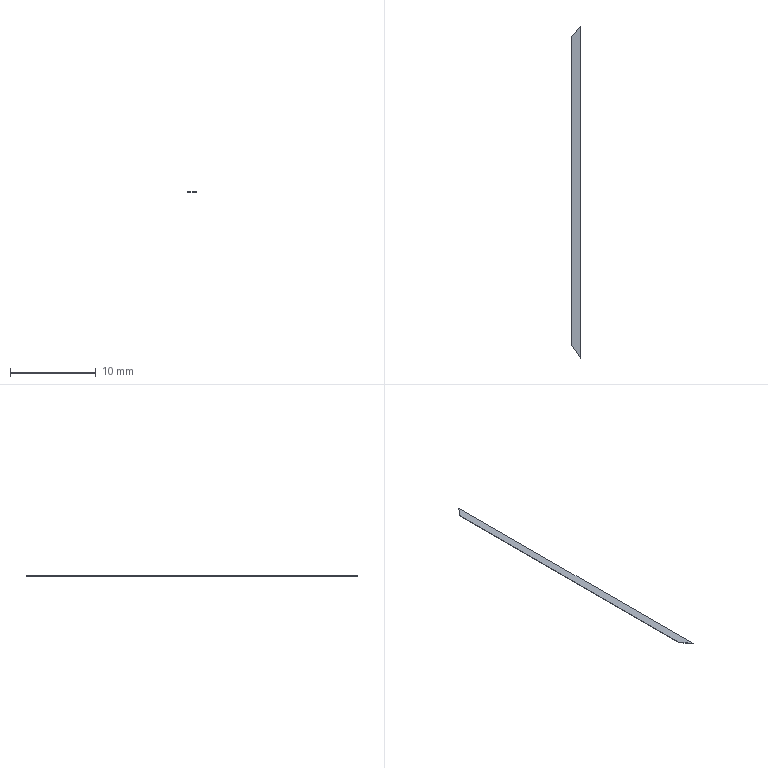Part | NX | features DATUM_CSYS 2, EXTRUDE 1, SKETCH 1 | 1 solid | 6 faces | box 1 x 38.63 x 0.05 mm | volume 1.865 mm3 | plane 6
STEP:
#1=CARTESIAN_POINT('',(0.,35.96,0.));
#2=VERTEX_POINT('',#1);
#3=CARTESIAN_POINT('',(0.,0.,0.));
#4=VERTEX_POINT('',#3);
#5=CARTESIAN_POINT('',(0.,35.96,0.));
#6=DIRECTION('',(0.,-1.,0.));
#7=VECTOR('',#6,1000.);
#8=LINE('',#5,#7);
#9=EDGE_CURVE('',#2,#4,#8,.T.);
#10=ORIENTED_EDGE('',*,*,#9,.T.);
#11=CARTESIAN_POINT('',(0.,0.,0.05));
#12=VERTEX_POINT('',#11);
#13=CARTESIAN_POINT('',(0.,0.,0.05));
#14=DIRECTION('',(0.,0.,-1.));
#15=VECTOR('',#14,1000.);
#16=LINE('',#13,#15);
#17=EDGE_CURVE('',#12,#4,#16,.T.);
#18=ORIENTED_EDGE('',*,*,#17,.F.);
#19=CARTESIAN_POINT('',(0.,35.96,0.05));
#20=VERTEX_POINT('',#19);
#21=CARTESIAN_POINT('',(0.,35.96,0.05));
#22=DIRECTION('',(0.,-1.,0.));
#23=VECTOR('',#22,1000.);
#24=LINE('',#21,#23);
#25=EDGE_CURVE('',#20,#12,#24,.T.);
#26=ORIENTED_EDGE('',*,*,#25,.F.);
#27=CARTESIAN_POINT('',(0.,35.96,0.05));
#28=DIRECTION('',(0.,0.,-1.));
#29=VECTOR('',#28,1000.);
#30=LINE('',#27,#29);
#31=EDGE_CURVE('',#20,#2,#30,.T.);
#32=ORIENTED_EDGE('',*,*,#31,.T.);
#33=EDGE_LOOP('',(#10,#18,#26,#32));
#34=FACE_BOUND('',#33,.T.);
#35=CARTESIAN_POINT('',(0.,35.96,0.05));
#36=DIRECTION('',(1.,0.,0.));
#37=DIRECTION('',(0.,0.,-1.));
#38=AXIS2_PLACEMENT_3D('',#35,#36,#37);
#39=PLANE('',#38);
#40=ADVANCED_FACE('',(#34),#39,.F.);
#41=CARTESIAN_POINT('',(1.,-1.41,0.));
#42=VERTEX_POINT('',#41);
#43=CARTESIAN_POINT('',(0.,0.,0.));
#44=DIRECTION('',(0.5785,-0.8157,0.));
#45=VECTOR('',#44,1000.);
#46=LINE('',#43,#45);
#47=EDGE_CURVE('',#4,#42,#46,.T.);
#48=ORIENTED_EDGE('',*,*,#47,.T.);
#49=CARTESIAN_POINT('',(1.,-1.41,0.05));
#50=VERTEX_POINT('',#49);
#51=CARTESIAN_POINT('',(1.,-1.41,0.05));
#52=DIRECTION('',(0.,0.,-1.));
#53=VECTOR('',#52,1000.);
#54=LINE('',#51,#53);
#55=EDGE_CURVE('',#50,#42,#54,.T.);
#56=ORIENTED_EDGE('',*,*,#55,.F.);
#57=CARTESIAN_POINT('',(0.,0.,0.05));
#58=DIRECTION('',(0.5785,-0.8157,0.));
#59=VECTOR('',#58,1000.);
#60=LINE('',#57,#59);
#61=EDGE_CURVE('',#12,#50,#60,.T.);
#62=ORIENTED_EDGE('',*,*,#61,.F.);
#63=ORIENTED_EDGE('',*,*,#17,.T.);
#64=EDGE_LOOP('',(#48,#56,#62,#63));
#65=FACE_BOUND('',#64,.T.);
#66=CARTESIAN_POINT('',(0.,0.,0.05));
#67=DIRECTION('',(0.8157,0.5785,0.));
#68=DIRECTION('',(-0.5785,0.8157,0.));
#69=AXIS2_PLACEMENT_3D('',#66,#67,#68);
#70=PLANE('',#69);
#71=ADVANCED_FACE('',(#65),#70,.F.);
#72=CARTESIAN_POINT('',(1.,37.22,0.));
#73=VERTEX_POINT('',#72);
#74=CARTESIAN_POINT('',(1.,-1.41,0.));
#75=DIRECTION('',(0.,1.,0.));
#76=VECTOR('',#75,1000.);
#77=LINE('',#74,#76);
#78=EDGE_CURVE('',#42,#73,#77,.T.);
#79=ORIENTED_EDGE('',*,*,#78,.T.);
#80=CARTESIAN_POINT('',(1.,37.22,0.05));
#81=VERTEX_POINT('',#80);
#82=CARTESIAN_POINT('',(1.,37.22,0.05));
#83=DIRECTION('',(0.,0.,-1.));
#84=VECTOR('',#83,1000.);
#85=LINE('',#82,#84);
#86=EDGE_CURVE('',#81,#73,#85,.T.);
#87=ORIENTED_EDGE('',*,*,#86,.F.);
#88=CARTESIAN_POINT('',(1.,-1.41,0.05));
#89=DIRECTION('',(0.,1.,0.));
#90=VECTOR('',#89,1000.);
#91=LINE('',#88,#90);
#92=EDGE_CURVE('',#50,#81,#91,.T.);
#93=ORIENTED_EDGE('',*,*,#92,.F.);
#94=ORIENTED_EDGE('',*,*,#55,.T.);
#95=EDGE_LOOP('',(#79,#87,#93,#94));
#96=FACE_BOUND('',#95,.T.);
#97=CARTESIAN_POINT('',(1.,-1.41,0.05));
#98=DIRECTION('',(-1.,0.,0.));
#99=DIRECTION('',(0.,-1.,0.));
#100=AXIS2_PLACEMENT_3D('',#97,#98,#99);
#101=PLANE('',#100);
#102=ADVANCED_FACE('',(#96),#101,.F.);
#103=CARTESIAN_POINT('',(1.,37.22,0.));
#104=DIRECTION('',(-0.6217,-0.7833,0.));
#105=VECTOR('',#104,1000.);
#106=LINE('',#103,#105);
#107=EDGE_CURVE('',#73,#2,#106,.T.);
#108=ORIENTED_EDGE('',*,*,#107,.T.);
#109=ORIENTED_EDGE('',*,*,#31,.F.);
#110=CARTESIAN_POINT('',(1.,37.22,0.05));
#111=DIRECTION('',(-0.6217,-0.7833,0.));
#112=VECTOR('',#111,1000.);
#113=LINE('',#110,#112);
#114=EDGE_CURVE('',#81,#20,#113,.T.);
#115=ORIENTED_EDGE('',*,*,#114,.F.);
#116=ORIENTED_EDGE('',*,*,#86,.T.);
#117=EDGE_LOOP('',(#108,#109,#115,#116));
#118=FACE_BOUND('',#117,.T.);
#119=CARTESIAN_POINT('',(1.,37.22,0.05));
#120=DIRECTION('',(0.7833,-0.6217,0.));
#121=DIRECTION('',(0.6217,0.7833,0.));
#122=AXIS2_PLACEMENT_3D('',#119,#120,#121);
#123=PLANE('',#122);
#124=ADVANCED_FACE('',(#118),#123,.F.);
#125=ORIENTED_EDGE('',*,*,#25,.T.);
#126=ORIENTED_EDGE('',*,*,#61,.T.);
#127=ORIENTED_EDGE('',*,*,#92,.T.);
#128=ORIENTED_EDGE('',*,*,#114,.T.);
#129=EDGE_LOOP('',(#125,#126,#127,#128));
#130=FACE_BOUND('',#129,.T.);
#131=CARTESIAN_POINT('',(0.,0.,0.05));
#132=DIRECTION('',(0.,0.,-1.));
#133=DIRECTION('',(-1.,0.,0.));
#134=AXIS2_PLACEMENT_3D('',#131,#132,#133);
#135=PLANE('',#134);
#136=ADVANCED_FACE('',(#130),#135,.F.);
#137=ORIENTED_EDGE('',*,*,#9,.F.);
#138=ORIENTED_EDGE('',*,*,#107,.F.);
#139=ORIENTED_EDGE('',*,*,#78,.F.);
#140=ORIENTED_EDGE('',*,*,#47,.F.);
#141=EDGE_LOOP('',(#137,#138,#139,#140));
#142=FACE_BOUND('',#141,.T.);
#143=CARTESIAN_POINT('',(0.,0.,0.));
#144=DIRECTION('',(0.,0.,-1.));
#145=DIRECTION('',(-1.,0.,0.));
#146=AXIS2_PLACEMENT_3D('',#143,#144,#145);
#147=PLANE('',#146);
#148=ADVANCED_FACE('',(#142),#147,.T.);
#149=CLOSED_SHELL('',(#40,#71,#102,#124,#136,#148));
#150=MANIFOLD_SOLID_BREP('',#149);
#151=(LENGTH_UNIT()NAMED_UNIT(*)SI_UNIT(.MILLI.,.METRE.));
#152=UNCERTAINTY_MEASURE_WITH_UNIT(LENGTH_MEASURE(0.00001),#151,'','');
#153=(NAMED_UNIT(*)PLANE_ANGLE_UNIT()SI_UNIT($,.RADIAN.));
#154=(NAMED_UNIT(*)SI_UNIT($,.STERADIAN.)SOLID_ANGLE_UNIT());
#155=(GEOMETRIC_REPRESENTATION_CONTEXT(3)GLOBAL_UNCERTAINTY_ASSIGNED_CONTEXT((#152))GLOBAL_UNIT_ASSIGNED_CONTEXT((#151,#153,#154))REPRESENTATION_CONTEXT('',''));
#156=ADVANCED_BREP_SHAPE_REPRESENTATION('',(#150),#155);